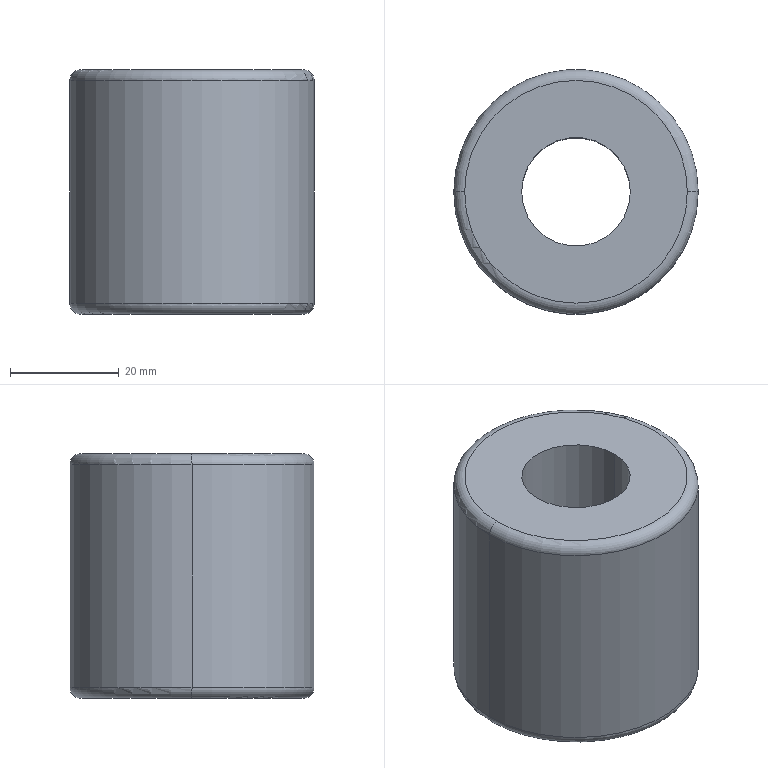Part | SolidWorks | features Extrusion 1, Fillet 1, ICE 1 | 1 solid | 10 faces | box 45 x 45 x 45 mm | volume 57194 mm3 | cylinder 4 | torus 4 | plane 2 | commonest cylinder face diameters 20 x2 45 x2
STEP:
#1=CARTESIAN_POINT('',(-10.,0.,0.));
#2=VERTEX_POINT('',#1);
#3=CARTESIAN_POINT('',(10.,0.,0.));
#4=VERTEX_POINT('',#3);
#5=CARTESIAN_POINT('',(0.,0.,0.));
#6=DIRECTION('',(0.,0.,1.));
#7=DIRECTION('',(1.,0.,0.));
#8=AXIS2_PLACEMENT_3D('',#5,#6,#7);
#9=CIRCLE('',#8,10.);
#10=EDGE_CURVE('',#2,#4,#9,.T.);
#11=ORIENTED_EDGE('',*,*,#10,.F.);
#12=CARTESIAN_POINT('',(-10.,0.,45.));
#13=VERTEX_POINT('',#12);
#14=CARTESIAN_POINT('',(-10.,0.,0.));
#15=DIRECTION('',(0.,0.,1.));
#16=VECTOR('',#15,1000.);
#17=LINE('',#14,#16);
#18=EDGE_CURVE('',#2,#13,#17,.T.);
#19=ORIENTED_EDGE('',*,*,#18,.T.);
#20=CARTESIAN_POINT('',(10.,0.,45.));
#21=VERTEX_POINT('',#20);
#22=CARTESIAN_POINT('',(0.,0.,45.));
#23=DIRECTION('',(0.,0.,1.));
#24=DIRECTION('',(1.,0.,0.));
#25=AXIS2_PLACEMENT_3D('',#22,#23,#24);
#26=CIRCLE('',#25,10.);
#27=EDGE_CURVE('',#13,#21,#26,.T.);
#28=ORIENTED_EDGE('',*,*,#27,.T.);
#29=CARTESIAN_POINT('',(10.,0.,0.));
#30=DIRECTION('',(0.,0.,1.));
#31=VECTOR('',#30,1000.);
#32=LINE('',#29,#31);
#33=EDGE_CURVE('',#4,#21,#32,.T.);
#34=ORIENTED_EDGE('',*,*,#33,.F.);
#35=EDGE_LOOP('',(#11,#19,#28,#34));
#36=FACE_OUTER_BOUND('',#35,.T.);
#37=CARTESIAN_POINT('',(0.,0.,0.));
#38=DIRECTION('',(0.,0.,1.));
#39=DIRECTION('',(1.,0.,0.));
#40=AXIS2_PLACEMENT_3D('',#37,#38,#39);
#41=CYLINDRICAL_SURFACE('',#40,10.);
#42=ADVANCED_FACE('',(#36),#41,.F.);
#43=CARTESIAN_POINT('',(-20.5,0.,0.));
#44=VERTEX_POINT('',#43);
#45=CARTESIAN_POINT('',(20.5,0.,0.));
#46=VERTEX_POINT('',#45);
#47=CARTESIAN_POINT('',(0.,0.,0.));
#48=DIRECTION('',(0.,0.,-1.));
#49=DIRECTION('',(1.,0.,0.));
#50=AXIS2_PLACEMENT_3D('',#47,#48,#49);
#51=CIRCLE('',#50,20.5);
#52=EDGE_CURVE('',#44,#46,#51,.T.);
#53=ORIENTED_EDGE('',*,*,#52,.F.);
#54=CARTESIAN_POINT('',(-22.5,0.,2.));
#55=VERTEX_POINT('',#54);
#56=CARTESIAN_POINT('',(-20.5,0.,2.));
#57=DIRECTION('',(0.,1.,0.));
#58=DIRECTION('',(-1.,0.,0.));
#59=AXIS2_PLACEMENT_3D('',#56,#57,#58);
#60=CIRCLE('',#59,2.);
#61=EDGE_CURVE('',#44,#55,#60,.T.);
#62=ORIENTED_EDGE('',*,*,#61,.T.);
#63=CARTESIAN_POINT('',(22.5,0.,2.));
#64=VERTEX_POINT('',#63);
#65=CARTESIAN_POINT('',(0.,0.,2.));
#66=DIRECTION('',(0.,0.,1.));
#67=DIRECTION('',(1.,0.,0.));
#68=AXIS2_PLACEMENT_3D('',#65,#66,#67);
#69=CIRCLE('',#68,22.5);
#70=EDGE_CURVE('',#64,#55,#69,.T.);
#71=ORIENTED_EDGE('',*,*,#70,.F.);
#72=CARTESIAN_POINT('',(20.5,0.,2.));
#73=DIRECTION('',(0.,-1.,0.));
#74=DIRECTION('',(0.,0.,-1.));
#75=AXIS2_PLACEMENT_3D('',#72,#73,#74);
#76=CIRCLE('',#75,2.);
#77=EDGE_CURVE('',#46,#64,#76,.T.);
#78=ORIENTED_EDGE('',*,*,#77,.F.);
#79=EDGE_LOOP('',(#53,#62,#71,#78));
#80=FACE_OUTER_BOUND('',#79,.T.);
#81=CARTESIAN_POINT('',(0.,0.,2.));
#82=DIRECTION('',(0.,0.,1.));
#83=DIRECTION('',(1.,0.,0.));
#84=AXIS2_PLACEMENT_3D('',#81,#82,#83);
#85=TOROIDAL_SURFACE('',#84,20.5,2.);
#86=ADVANCED_FACE('',(#80),#85,.T.);
#87=CARTESIAN_POINT('',(-22.5,0.,43.));
#88=VERTEX_POINT('',#87);
#89=CARTESIAN_POINT('',(22.5,0.,43.));
#90=VERTEX_POINT('',#89);
#91=CARTESIAN_POINT('',(0.,0.,43.));
#92=DIRECTION('',(0.,0.,-1.));
#93=DIRECTION('',(1.,0.,0.));
#94=AXIS2_PLACEMENT_3D('',#91,#92,#93);
#95=CIRCLE('',#94,22.5);
#96=EDGE_CURVE('',#88,#90,#95,.T.);
#97=ORIENTED_EDGE('',*,*,#96,.F.);
#98=CARTESIAN_POINT('',(-20.5,0.,45.));
#99=VERTEX_POINT('',#98);
#100=CARTESIAN_POINT('',(-20.5,0.,43.));
#101=DIRECTION('',(0.,1.,0.));
#102=DIRECTION('',(-1.,0.,0.));
#103=AXIS2_PLACEMENT_3D('',#100,#101,#102);
#104=CIRCLE('',#103,2.);
#105=EDGE_CURVE('',#88,#99,#104,.T.);
#106=ORIENTED_EDGE('',*,*,#105,.T.);
#107=CARTESIAN_POINT('',(20.5,0.,45.));
#108=VERTEX_POINT('',#107);
#109=CARTESIAN_POINT('',(0.,0.,45.));
#110=DIRECTION('',(0.,0.,1.));
#111=DIRECTION('',(1.,0.,0.));
#112=AXIS2_PLACEMENT_3D('',#109,#110,#111);
#113=CIRCLE('',#112,20.5);
#114=EDGE_CURVE('',#108,#99,#113,.T.);
#115=ORIENTED_EDGE('',*,*,#114,.F.);
#116=CARTESIAN_POINT('',(20.5,0.,43.));
#117=DIRECTION('',(0.,-1.,0.));
#118=DIRECTION('',(0.,0.,-1.));
#119=AXIS2_PLACEMENT_3D('',#116,#117,#118);
#120=CIRCLE('',#119,2.);
#121=EDGE_CURVE('',#90,#108,#120,.T.);
#122=ORIENTED_EDGE('',*,*,#121,.F.);
#123=EDGE_LOOP('',(#97,#106,#115,#122));
#124=FACE_OUTER_BOUND('',#123,.T.);
#125=CARTESIAN_POINT('',(0.,0.,43.));
#126=DIRECTION('',(0.,0.,1.));
#127=DIRECTION('',(1.,0.,0.));
#128=AXIS2_PLACEMENT_3D('',#125,#126,#127);
#129=TOROIDAL_SURFACE('',#128,20.5,2.);
#130=ADVANCED_FACE('',(#124),#129,.T.);
#131=ORIENTED_EDGE('',*,*,#96,.T.);
#132=CARTESIAN_POINT('',(22.5,0.,45.));
#133=DIRECTION('',(0.,0.,-1.));
#134=VECTOR('',#133,1000.);
#135=LINE('',#132,#134);
#136=EDGE_CURVE('',#90,#64,#135,.T.);
#137=ORIENTED_EDGE('',*,*,#136,.T.);
#138=ORIENTED_EDGE('',*,*,#70,.T.);
#139=CARTESIAN_POINT('',(-22.5,0.,45.));
#140=DIRECTION('',(0.,0.,-1.));
#141=VECTOR('',#140,1000.);
#142=LINE('',#139,#141);
#143=EDGE_CURVE('',#88,#55,#142,.T.);
#144=ORIENTED_EDGE('',*,*,#143,.F.);
#145=EDGE_LOOP('',(#131,#137,#138,#144));
#146=FACE_OUTER_BOUND('',#145,.T.);
#147=CARTESIAN_POINT('',(0.,0.,45.));
#148=DIRECTION('',(0.,0.,-1.));
#149=DIRECTION('',(-1.,0.,0.));
#150=AXIS2_PLACEMENT_3D('',#147,#148,#149);
#151=CYLINDRICAL_SURFACE('',#150,22.5);
#152=ADVANCED_FACE('',(#146),#151,.T.);
#153=ORIENTED_EDGE('',*,*,#136,.F.);
#154=CARTESIAN_POINT('',(0.,0.,43.));
#155=DIRECTION('',(0.,0.,-1.));
#156=DIRECTION('',(1.,0.,0.));
#157=AXIS2_PLACEMENT_3D('',#154,#155,#156);
#158=CIRCLE('',#157,22.5);
#159=EDGE_CURVE('',#90,#88,#158,.T.);
#160=ORIENTED_EDGE('',*,*,#159,.T.);
#161=ORIENTED_EDGE('',*,*,#143,.T.);
#162=CARTESIAN_POINT('',(0.,0.,2.));
#163=DIRECTION('',(0.,0.,1.));
#164=DIRECTION('',(1.,0.,0.));
#165=AXIS2_PLACEMENT_3D('',#162,#163,#164);
#166=CIRCLE('',#165,22.5);
#167=EDGE_CURVE('',#55,#64,#166,.T.);
#168=ORIENTED_EDGE('',*,*,#167,.T.);
#169=EDGE_LOOP('',(#153,#160,#161,#168));
#170=FACE_OUTER_BOUND('',#169,.T.);
#171=CARTESIAN_POINT('',(0.,0.,45.));
#172=DIRECTION('',(0.,0.,-1.));
#173=DIRECTION('',(-1.,0.,0.));
#174=AXIS2_PLACEMENT_3D('',#171,#172,#173);
#175=CYLINDRICAL_SURFACE('',#174,22.5);
#176=ADVANCED_FACE('',(#170),#175,.T.);
#177=CARTESIAN_POINT('',(0.,0.,45.));
#178=DIRECTION('',(0.,0.,1.));
#179=DIRECTION('',(1.,0.,0.));
#180=AXIS2_PLACEMENT_3D('',#177,#178,#179);
#181=CIRCLE('',#180,10.);
#182=EDGE_CURVE('',#21,#13,#181,.T.);
#183=ORIENTED_EDGE('',*,*,#182,.F.);
#184=ORIENTED_EDGE('',*,*,#27,.F.);
#185=EDGE_LOOP('',(#183,#184));
#186=FACE_BOUND('',#185,.T.);
#187=ORIENTED_EDGE('',*,*,#114,.T.);
#188=CARTESIAN_POINT('',(0.,0.,45.));
#189=DIRECTION('',(0.,0.,1.));
#190=DIRECTION('',(1.,0.,0.));
#191=AXIS2_PLACEMENT_3D('',#188,#189,#190);
#192=CIRCLE('',#191,20.5);
#193=EDGE_CURVE('',#99,#108,#192,.T.);
#194=ORIENTED_EDGE('',*,*,#193,.T.);
#195=EDGE_LOOP('',(#187,#194));
#196=FACE_OUTER_BOUND('',#195,.T.);
#197=CARTESIAN_POINT('',(0.,0.,45.));
#198=DIRECTION('',(0.,0.,1.));
#199=DIRECTION('',(1.,0.,0.));
#200=AXIS2_PLACEMENT_3D('',#197,#198,#199);
#201=PLANE('',#200);
#202=ADVANCED_FACE('',(#186,#196),#201,.T.);
#203=CARTESIAN_POINT('',(0.,0.,0.));
#204=DIRECTION('',(0.,0.,1.));
#205=DIRECTION('',(1.,0.,0.));
#206=AXIS2_PLACEMENT_3D('',#203,#204,#205);
#207=CIRCLE('',#206,10.);
#208=EDGE_CURVE('',#4,#2,#207,.T.);
#209=ORIENTED_EDGE('',*,*,#208,.T.);
#210=ORIENTED_EDGE('',*,*,#10,.T.);
#211=EDGE_LOOP('',(#209,#210));
#212=FACE_BOUND('',#211,.T.);
#213=CARTESIAN_POINT('',(0.,0.,0.));
#214=DIRECTION('',(0.,0.,-1.));
#215=DIRECTION('',(1.,0.,0.));
#216=AXIS2_PLACEMENT_3D('',#213,#214,#215);
#217=CIRCLE('',#216,20.5);
#218=EDGE_CURVE('',#46,#44,#217,.T.);
#219=ORIENTED_EDGE('',*,*,#218,.T.);
#220=ORIENTED_EDGE('',*,*,#52,.T.);
#221=EDGE_LOOP('',(#219,#220));
#222=FACE_OUTER_BOUND('',#221,.T.);
#223=CARTESIAN_POINT('',(0.,0.,0.));
#224=DIRECTION('',(0.,0.,1.));
#225=DIRECTION('',(1.,0.,0.));
#226=AXIS2_PLACEMENT_3D('',#223,#224,#225);
#227=PLANE('',#226);
#228=ADVANCED_FACE('',(#212,#222),#227,.F.);
#229=ORIENTED_EDGE('',*,*,#105,.F.);
#230=ORIENTED_EDGE('',*,*,#159,.F.);
#231=ORIENTED_EDGE('',*,*,#121,.T.);
#232=ORIENTED_EDGE('',*,*,#193,.F.);
#233=EDGE_LOOP('',(#229,#230,#231,#232));
#234=FACE_OUTER_BOUND('',#233,.T.);
#235=CARTESIAN_POINT('',(0.,0.,43.));
#236=DIRECTION('',(0.,0.,1.));
#237=DIRECTION('',(1.,0.,0.));
#238=AXIS2_PLACEMENT_3D('',#235,#236,#237);
#239=TOROIDAL_SURFACE('',#238,20.5,2.);
#240=ADVANCED_FACE('',(#234),#239,.T.);
#241=ORIENTED_EDGE('',*,*,#61,.F.);
#242=ORIENTED_EDGE('',*,*,#218,.F.);
#243=ORIENTED_EDGE('',*,*,#77,.T.);
#244=ORIENTED_EDGE('',*,*,#167,.F.);
#245=EDGE_LOOP('',(#241,#242,#243,#244));
#246=FACE_OUTER_BOUND('',#245,.T.);
#247=CARTESIAN_POINT('',(0.,0.,2.));
#248=DIRECTION('',(0.,0.,1.));
#249=DIRECTION('',(1.,0.,0.));
#250=AXIS2_PLACEMENT_3D('',#247,#248,#249);
#251=TOROIDAL_SURFACE('',#250,20.5,2.);
#252=ADVANCED_FACE('',(#246),#251,.T.);
#253=ORIENTED_EDGE('',*,*,#18,.F.);
#254=ORIENTED_EDGE('',*,*,#208,.F.);
#255=ORIENTED_EDGE('',*,*,#33,.T.);
#256=ORIENTED_EDGE('',*,*,#182,.T.);
#257=EDGE_LOOP('',(#253,#254,#255,#256));
#258=FACE_OUTER_BOUND('',#257,.T.);
#259=CARTESIAN_POINT('',(0.,0.,0.));
#260=DIRECTION('',(0.,0.,1.));
#261=DIRECTION('',(1.,0.,0.));
#262=AXIS2_PLACEMENT_3D('',#259,#260,#261);
#263=CYLINDRICAL_SURFACE('',#262,10.);
#264=ADVANCED_FACE('',(#258),#263,.F.);
#265=CLOSED_SHELL('',(#42,#86,#130,#152,#176,#202,#228,#240,#252,#264));
#266=MANIFOLD_SOLID_BREP('',#265);
#267=CARTESIAN_POINT('',(0.,0.,0.));
#268=DIRECTION('',(0.,0.,1.));
#269=DIRECTION('',(1.,0.,0.));
#270=AXIS2_PLACEMENT_3D('',#267,#268,#269);
#271=(LENGTH_UNIT()NAMED_UNIT(*)SI_UNIT(.MILLI.,.METRE.));
#272=UNCERTAINTY_MEASURE_WITH_UNIT(LENGTH_MEASURE(0.00001),#271,'','');
#273=(NAMED_UNIT(*)PLANE_ANGLE_UNIT()SI_UNIT($,.RADIAN.));
#274=(NAMED_UNIT(*)SI_UNIT($,.STERADIAN.)SOLID_ANGLE_UNIT());
#275=(GEOMETRIC_REPRESENTATION_CONTEXT(3)GLOBAL_UNCERTAINTY_ASSIGNED_CONTEXT((#272))GLOBAL_UNIT_ASSIGNED_CONTEXT((#271,#273,#274))REPRESENTATION_CONTEXT('',''));
#276=ADVANCED_BREP_SHAPE_REPRESENTATION('',(#266,#270),#275);